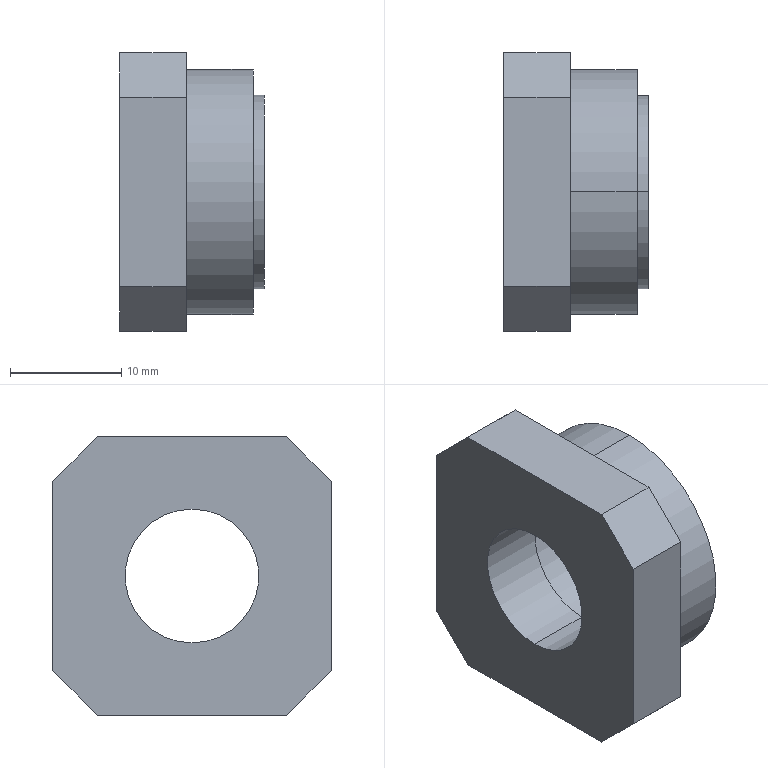Part | SolidWorks | features ICE 2, Chamfer 1, Extrusion 1, HoleWzd 1 | 1 solid | 21 faces | box 13 x 25 x 25 mm | volume 4305 mm3 | plane 13 | cylinder 8 | commonest cylinder face diameters 12 x2 14.1 x2 17.4 x2 22 x2
STEP:
#1=CARTESIAN_POINT('',(9.,0.,-8.7));
#2=VERTEX_POINT('',#1);
#3=CARTESIAN_POINT('',(9.,0.,8.7));
#4=VERTEX_POINT('',#3);
#5=CARTESIAN_POINT('',(9.,0.,0.));
#6=DIRECTION('',(1.,0.,0.));
#7=DIRECTION('',(0.,0.,-1.));
#8=AXIS2_PLACEMENT_3D('',#5,#6,#7);
#9=CIRCLE('',#8,8.7);
#10=EDGE_CURVE('',#2,#4,#9,.T.);
#11=ORIENTED_EDGE('',*,*,#10,.T.);
#12=CARTESIAN_POINT('',(10.,0.,8.7));
#13=VERTEX_POINT('',#12);
#14=CARTESIAN_POINT('',(9.,0.,8.7));
#15=DIRECTION('',(1.,0.,0.));
#16=VECTOR('',#15,1000.);
#17=LINE('',#14,#16);
#18=EDGE_CURVE('',#4,#13,#17,.T.);
#19=ORIENTED_EDGE('',*,*,#18,.T.);
#20=CARTESIAN_POINT('',(10.,0.,-8.7));
#21=VERTEX_POINT('',#20);
#22=CARTESIAN_POINT('',(10.,0.,0.));
#23=DIRECTION('',(1.,0.,0.));
#24=DIRECTION('',(0.,0.,-1.));
#25=AXIS2_PLACEMENT_3D('',#22,#23,#24);
#26=CIRCLE('',#25,8.7);
#27=EDGE_CURVE('',#21,#13,#26,.T.);
#28=ORIENTED_EDGE('',*,*,#27,.F.);
#29=CARTESIAN_POINT('',(9.,0.,-8.7));
#30=DIRECTION('',(1.,0.,0.));
#31=VECTOR('',#30,1000.);
#32=LINE('',#29,#31);
#33=EDGE_CURVE('',#2,#21,#32,.T.);
#34=ORIENTED_EDGE('',*,*,#33,.F.);
#35=EDGE_LOOP('',(#11,#19,#28,#34));
#36=FACE_OUTER_BOUND('',#35,.T.);
#37=CARTESIAN_POINT('',(9.,0.,0.));
#38=DIRECTION('',(1.,0.,0.));
#39=DIRECTION('',(0.,0.,-1.));
#40=AXIS2_PLACEMENT_3D('',#37,#38,#39);
#41=CYLINDRICAL_SURFACE('',#40,8.7);
#42=ADVANCED_FACE('',(#36),#41,.T.);
#43=CARTESIAN_POINT('',(10.,0.,7.05));
#44=VERTEX_POINT('',#43);
#45=CARTESIAN_POINT('',(10.,0.,-7.05));
#46=VERTEX_POINT('',#45);
#47=CARTESIAN_POINT('',(10.,0.,0.));
#48=DIRECTION('',(1.,0.,0.));
#49=DIRECTION('',(0.,0.,-1.));
#50=AXIS2_PLACEMENT_3D('',#47,#48,#49);
#51=CIRCLE('',#50,7.05);
#52=EDGE_CURVE('',#44,#46,#51,.T.);
#53=ORIENTED_EDGE('',*,*,#52,.T.);
#54=CARTESIAN_POINT('',(3.,0.,-7.05));
#55=VERTEX_POINT('',#54);
#56=CARTESIAN_POINT('',(10.,0.,-7.05));
#57=DIRECTION('',(-1.,0.,0.));
#58=VECTOR('',#57,1000.);
#59=LINE('',#56,#58);
#60=EDGE_CURVE('',#46,#55,#59,.T.);
#61=ORIENTED_EDGE('',*,*,#60,.T.);
#62=CARTESIAN_POINT('',(3.,0.,7.05));
#63=VERTEX_POINT('',#62);
#64=CARTESIAN_POINT('',(3.,0.,0.));
#65=DIRECTION('',(1.,0.,0.));
#66=DIRECTION('',(0.,0.,-1.));
#67=AXIS2_PLACEMENT_3D('',#64,#65,#66);
#68=CIRCLE('',#67,7.05);
#69=EDGE_CURVE('',#63,#55,#68,.T.);
#70=ORIENTED_EDGE('',*,*,#69,.F.);
#71=CARTESIAN_POINT('',(10.,0.,7.05));
#72=DIRECTION('',(-1.,0.,0.));
#73=VECTOR('',#72,1000.);
#74=LINE('',#71,#73);
#75=EDGE_CURVE('',#44,#63,#74,.T.);
#76=ORIENTED_EDGE('',*,*,#75,.F.);
#77=EDGE_LOOP('',(#53,#61,#70,#76));
#78=FACE_OUTER_BOUND('',#77,.T.);
#79=CARTESIAN_POINT('',(10.,0.,0.));
#80=DIRECTION('',(-1.,0.,0.));
#81=DIRECTION('',(0.,0.,1.));
#82=AXIS2_PLACEMENT_3D('',#79,#80,#81);
#83=CYLINDRICAL_SURFACE('',#82,7.05);
#84=ADVANCED_FACE('',(#78),#83,.F.);
#85=CARTESIAN_POINT('',(3.,0.,-6.));
#86=VERTEX_POINT('',#85);
#87=CARTESIAN_POINT('',(3.,0.,6.));
#88=VERTEX_POINT('',#87);
#89=CARTESIAN_POINT('',(3.,0.,0.));
#90=DIRECTION('',(-1.,0.,0.));
#91=DIRECTION('',(0.,0.,1.));
#92=AXIS2_PLACEMENT_3D('',#89,#90,#91);
#93=CIRCLE('',#92,6.);
#94=EDGE_CURVE('',#86,#88,#93,.T.);
#95=ORIENTED_EDGE('',*,*,#94,.F.);
#96=CARTESIAN_POINT('',(-3.,0.,-6.));
#97=VERTEX_POINT('',#96);
#98=CARTESIAN_POINT('',(-3.,0.,-6.));
#99=DIRECTION('',(-1.,0.,0.));
#100=VECTOR('',#99,1000.);
#101=LINE('',#98,#100);
#102=EDGE_CURVE('',#86,#97,#101,.T.);
#103=ORIENTED_EDGE('',*,*,#102,.T.);
#104=CARTESIAN_POINT('',(-3.,0.,6.));
#105=VERTEX_POINT('',#104);
#106=CARTESIAN_POINT('',(-3.,0.,0.));
#107=DIRECTION('',(-1.,0.,0.));
#108=DIRECTION('',(0.,0.,1.));
#109=AXIS2_PLACEMENT_3D('',#106,#107,#108);
#110=CIRCLE('',#109,6.);
#111=EDGE_CURVE('',#97,#105,#110,.T.);
#112=ORIENTED_EDGE('',*,*,#111,.T.);
#113=CARTESIAN_POINT('',(-3.,0.,6.));
#114=DIRECTION('',(-1.,0.,0.));
#115=VECTOR('',#114,1000.);
#116=LINE('',#113,#115);
#117=EDGE_CURVE('',#88,#105,#116,.T.);
#118=ORIENTED_EDGE('',*,*,#117,.F.);
#119=EDGE_LOOP('',(#95,#103,#112,#118));
#120=FACE_OUTER_BOUND('',#119,.T.);
#121=CARTESIAN_POINT('',(-3.,0.,0.));
#122=DIRECTION('',(-1.,0.,0.));
#123=DIRECTION('',(0.,0.,1.));
#124=AXIS2_PLACEMENT_3D('',#121,#122,#123);
#125=CYLINDRICAL_SURFACE('',#124,6.);
#126=ADVANCED_FACE('',(#120),#125,.F.);
#127=CARTESIAN_POINT('',(9.,0.,-11.));
#128=VERTEX_POINT('',#127);
#129=CARTESIAN_POINT('',(9.,0.,11.));
#130=VERTEX_POINT('',#129);
#131=CARTESIAN_POINT('',(9.,0.,0.));
#132=DIRECTION('',(1.,0.,0.));
#133=DIRECTION('',(0.,0.,-1.));
#134=AXIS2_PLACEMENT_3D('',#131,#132,#133);
#135=CIRCLE('',#134,11.);
#136=EDGE_CURVE('',#128,#130,#135,.T.);
#137=ORIENTED_EDGE('',*,*,#136,.F.);
#138=CARTESIAN_POINT('',(3.,0.,-11.));
#139=VERTEX_POINT('',#138);
#140=CARTESIAN_POINT('',(10.,0.,-11.));
#141=DIRECTION('',(-1.,0.,0.));
#142=VECTOR('',#141,1000.);
#143=LINE('',#140,#142);
#144=EDGE_CURVE('',#128,#139,#143,.T.);
#145=ORIENTED_EDGE('',*,*,#144,.T.);
#146=CARTESIAN_POINT('',(3.,0.,11.));
#147=VERTEX_POINT('',#146);
#148=CARTESIAN_POINT('',(3.,0.,0.));
#149=DIRECTION('',(1.,0.,0.));
#150=DIRECTION('',(0.,0.,-1.));
#151=AXIS2_PLACEMENT_3D('',#148,#149,#150);
#152=CIRCLE('',#151,11.);
#153=EDGE_CURVE('',#139,#147,#152,.T.);
#154=ORIENTED_EDGE('',*,*,#153,.T.);
#155=CARTESIAN_POINT('',(10.,0.,11.));
#156=DIRECTION('',(-1.,0.,0.));
#157=VECTOR('',#156,1000.);
#158=LINE('',#155,#157);
#159=EDGE_CURVE('',#130,#147,#158,.T.);
#160=ORIENTED_EDGE('',*,*,#159,.F.);
#161=EDGE_LOOP('',(#137,#145,#154,#160));
#162=FACE_OUTER_BOUND('',#161,.T.);
#163=CARTESIAN_POINT('',(10.,0.,0.));
#164=DIRECTION('',(-1.,0.,0.));
#165=DIRECTION('',(0.,0.,1.));
#166=AXIS2_PLACEMENT_3D('',#163,#164,#165);
#167=CYLINDRICAL_SURFACE('',#166,11.);
#168=ADVANCED_FACE('',(#162),#167,.T.);
#169=ORIENTED_EDGE('',*,*,#52,.F.);
#170=CARTESIAN_POINT('',(10.,0.,0.));
#171=DIRECTION('',(1.,0.,0.));
#172=DIRECTION('',(0.,0.,-1.));
#173=AXIS2_PLACEMENT_3D('',#170,#171,#172);
#174=CIRCLE('',#173,7.05);
#175=EDGE_CURVE('',#46,#44,#174,.T.);
#176=ORIENTED_EDGE('',*,*,#175,.F.);
#177=EDGE_LOOP('',(#169,#176));
#178=FACE_BOUND('',#177,.T.);
#179=ORIENTED_EDGE('',*,*,#27,.T.);
#180=CARTESIAN_POINT('',(10.,0.,0.));
#181=DIRECTION('',(1.,0.,0.));
#182=DIRECTION('',(0.,0.,-1.));
#183=AXIS2_PLACEMENT_3D('',#180,#181,#182);
#184=CIRCLE('',#183,8.7);
#185=EDGE_CURVE('',#13,#21,#184,.T.);
#186=ORIENTED_EDGE('',*,*,#185,.T.);
#187=EDGE_LOOP('',(#179,#186));
#188=FACE_OUTER_BOUND('',#187,.T.);
#189=CARTESIAN_POINT('',(10.,0.,0.));
#190=DIRECTION('',(1.,0.,0.));
#191=DIRECTION('',(0.,0.,-1.));
#192=AXIS2_PLACEMENT_3D('',#189,#190,#191);
#193=PLANE('',#192);
#194=ADVANCED_FACE('',(#178,#188),#193,.T.);
#195=ORIENTED_EDGE('',*,*,#144,.F.);
#196=CARTESIAN_POINT('',(9.,0.,0.));
#197=DIRECTION('',(1.,0.,0.));
#198=DIRECTION('',(0.,0.,-1.));
#199=AXIS2_PLACEMENT_3D('',#196,#197,#198);
#200=CIRCLE('',#199,11.);
#201=EDGE_CURVE('',#130,#128,#200,.T.);
#202=ORIENTED_EDGE('',*,*,#201,.F.);
#203=ORIENTED_EDGE('',*,*,#159,.T.);
#204=CARTESIAN_POINT('',(3.,0.,0.));
#205=DIRECTION('',(1.,0.,0.));
#206=DIRECTION('',(0.,0.,-1.));
#207=AXIS2_PLACEMENT_3D('',#204,#205,#206);
#208=CIRCLE('',#207,11.);
#209=EDGE_CURVE('',#147,#139,#208,.T.);
#210=ORIENTED_EDGE('',*,*,#209,.T.);
#211=EDGE_LOOP('',(#195,#202,#203,#210));
#212=FACE_OUTER_BOUND('',#211,.T.);
#213=CARTESIAN_POINT('',(10.,0.,0.));
#214=DIRECTION('',(-1.,0.,0.));
#215=DIRECTION('',(0.,0.,1.));
#216=AXIS2_PLACEMENT_3D('',#213,#214,#215);
#217=CYLINDRICAL_SURFACE('',#216,11.);
#218=ADVANCED_FACE('',(#212),#217,.T.);
#219=CARTESIAN_POINT('',(3.,0.,0.));
#220=DIRECTION('',(-1.,0.,0.));
#221=DIRECTION('',(0.,0.,1.));
#222=AXIS2_PLACEMENT_3D('',#219,#220,#221);
#223=CIRCLE('',#222,6.);
#224=EDGE_CURVE('',#88,#86,#223,.T.);
#225=ORIENTED_EDGE('',*,*,#224,.T.);
#226=ORIENTED_EDGE('',*,*,#94,.T.);
#227=EDGE_LOOP('',(#225,#226));
#228=FACE_BOUND('',#227,.T.);
#229=ORIENTED_EDGE('',*,*,#69,.T.);
#230=CARTESIAN_POINT('',(3.,0.,0.));
#231=DIRECTION('',(1.,0.,0.));
#232=DIRECTION('',(0.,0.,-1.));
#233=AXIS2_PLACEMENT_3D('',#230,#231,#232);
#234=CIRCLE('',#233,7.05);
#235=EDGE_CURVE('',#55,#63,#234,.T.);
#236=ORIENTED_EDGE('',*,*,#235,.T.);
#237=EDGE_LOOP('',(#229,#236));
#238=FACE_OUTER_BOUND('',#237,.T.);
#239=CARTESIAN_POINT('',(3.,0.,0.));
#240=DIRECTION('',(-1.,0.,0.));
#241=DIRECTION('',(0.,0.,1.));
#242=AXIS2_PLACEMENT_3D('',#239,#240,#241);
#243=PLANE('',#242);
#244=ADVANCED_FACE('',(#228,#238),#243,.F.);
#245=CARTESIAN_POINT('',(3.,-8.5,-12.5));
#246=VERTEX_POINT('',#245);
#247=CARTESIAN_POINT('',(3.,8.5,-12.5));
#248=VERTEX_POINT('',#247);
#249=CARTESIAN_POINT('',(3.,-12.5,-12.5));
#250=DIRECTION('',(0.,1.,0.));
#251=VECTOR('',#250,1000.);
#252=LINE('',#249,#251);
#253=EDGE_CURVE('',#246,#248,#252,.T.);
#254=ORIENTED_EDGE('',*,*,#253,.F.);
#255=CARTESIAN_POINT('',(-3.,-8.5,-12.5));
#256=VERTEX_POINT('',#255);
#257=CARTESIAN_POINT('',(3.,-8.5,-12.5));
#258=DIRECTION('',(-1.,0.,0.));
#259=VECTOR('',#258,1000.);
#260=LINE('',#257,#259);
#261=EDGE_CURVE('',#246,#256,#260,.T.);
#262=ORIENTED_EDGE('',*,*,#261,.T.);
#263=CARTESIAN_POINT('',(-3.,8.5,-12.5));
#264=VERTEX_POINT('',#263);
#265=CARTESIAN_POINT('',(-3.,-12.5,-12.5));
#266=DIRECTION('',(0.,1.,0.));
#267=VECTOR('',#266,1000.);
#268=LINE('',#265,#267);
#269=EDGE_CURVE('',#256,#264,#268,.T.);
#270=ORIENTED_EDGE('',*,*,#269,.T.);
#271=CARTESIAN_POINT('',(3.,8.5,-12.5));
#272=DIRECTION('',(1.,0.,0.));
#273=VECTOR('',#272,1000.);
#274=LINE('',#271,#273);
#275=EDGE_CURVE('',#264,#248,#274,.T.);
#276=ORIENTED_EDGE('',*,*,#275,.T.);
#277=EDGE_LOOP('',(#254,#262,#270,#276));
#278=FACE_OUTER_BOUND('',#277,.T.);
#279=CARTESIAN_POINT('',(3.,-12.5,-12.5));
#280=DIRECTION('',(0.,0.,1.));
#281=DIRECTION('',(1.,0.,0.));
#282=AXIS2_PLACEMENT_3D('',#279,#280,#281);
#283=PLANE('',#282);
#284=ADVANCED_FACE('',(#278),#283,.F.);
#285=CARTESIAN_POINT('',(3.,12.5,-8.5));
#286=VERTEX_POINT('',#285);
#287=CARTESIAN_POINT('',(3.,12.5,8.5));
#288=VERTEX_POINT('',#287);
#289=CARTESIAN_POINT('',(3.,12.5,12.5));
#290=DIRECTION('',(0.,0.,1.));
#291=VECTOR('',#290,1000.);
#292=LINE('',#289,#291);
#293=EDGE_CURVE('',#286,#288,#292,.T.);
#294=ORIENTED_EDGE('',*,*,#293,.F.);
#295=CARTESIAN_POINT('',(-3.,12.5,-8.5));
#296=VERTEX_POINT('',#295);
#297=CARTESIAN_POINT('',(3.,12.5,-8.5));
#298=DIRECTION('',(-1.,0.,0.));
#299=VECTOR('',#298,1000.);
#300=LINE('',#297,#299);
#301=EDGE_CURVE('',#286,#296,#300,.T.);
#302=ORIENTED_EDGE('',*,*,#301,.T.);
#303=CARTESIAN_POINT('',(-3.,12.5,8.5));
#304=VERTEX_POINT('',#303);
#305=CARTESIAN_POINT('',(-3.,12.5,12.5));
#306=DIRECTION('',(0.,0.,1.));
#307=VECTOR('',#306,1000.);
#308=LINE('',#305,#307);
#309=EDGE_CURVE('',#296,#304,#308,.T.);
#310=ORIENTED_EDGE('',*,*,#309,.T.);
#311=CARTESIAN_POINT('',(3.,12.5,8.5));
#312=DIRECTION('',(1.,0.,0.));
#313=VECTOR('',#312,1000.);
#314=LINE('',#311,#313);
#315=EDGE_CURVE('',#304,#288,#314,.T.);
#316=ORIENTED_EDGE('',*,*,#315,.T.);
#317=EDGE_LOOP('',(#294,#302,#310,#316));
#318=FACE_OUTER_BOUND('',#317,.T.);
#319=CARTESIAN_POINT('',(3.,12.5,12.5));
#320=DIRECTION('',(0.,-1.,0.));
#321=DIRECTION('',(0.,0.,-1.));
#322=AXIS2_PLACEMENT_3D('',#319,#320,#321);
#323=PLANE('',#322);
#324=ADVANCED_FACE('',(#318),#323,.F.);
#325=CARTESIAN_POINT('',(-3.,8.5,12.5));
#326=VERTEX_POINT('',#325);
#327=CARTESIAN_POINT('',(-3.,-8.5,12.5));
#328=VERTEX_POINT('',#327);
#329=CARTESIAN_POINT('',(-3.,-12.5,12.5));
#330=DIRECTION('',(0.,-1.,0.));
#331=VECTOR('',#330,1000.);
#332=LINE('',#329,#331);
#333=EDGE_CURVE('',#326,#328,#332,.T.);
#334=ORIENTED_EDGE('',*,*,#333,.T.);
#335=CARTESIAN_POINT('',(3.,-8.5,12.5));
#336=VERTEX_POINT('',#335);
#337=CARTESIAN_POINT('',(3.,-8.5,12.5));
#338=DIRECTION('',(1.,0.,0.));
#339=VECTOR('',#338,1000.);
#340=LINE('',#337,#339);
#341=EDGE_CURVE('',#328,#336,#340,.T.);
#342=ORIENTED_EDGE('',*,*,#341,.T.);
#343=CARTESIAN_POINT('',(3.,8.5,12.5));
#344=VERTEX_POINT('',#343);
#345=CARTESIAN_POINT('',(3.,-12.5,12.5));
#346=DIRECTION('',(0.,-1.,0.));
#347=VECTOR('',#346,1000.);
#348=LINE('',#345,#347);
#349=EDGE_CURVE('',#344,#336,#348,.T.);
#350=ORIENTED_EDGE('',*,*,#349,.F.);
#351=CARTESIAN_POINT('',(3.,8.5,12.5));
#352=DIRECTION('',(-1.,0.,0.));
#353=VECTOR('',#352,1000.);
#354=LINE('',#351,#353);
#355=EDGE_CURVE('',#344,#326,#354,.T.);
#356=ORIENTED_EDGE('',*,*,#355,.T.);
#357=EDGE_LOOP('',(#334,#342,#350,#356));
#358=FACE_OUTER_BOUND('',#357,.T.);
#359=CARTESIAN_POINT('',(3.,-12.5,12.5));
#360=DIRECTION('',(0.,0.,-1.));
#361=DIRECTION('',(-1.,0.,0.));
#362=AXIS2_PLACEMENT_3D('',#359,#360,#361);
#363=PLANE('',#362);
#364=ADVANCED_FACE('',(#358),#363,.F.);
#365=CARTESIAN_POINT('',(3.,-12.5,8.5));
#366=VERTEX_POINT('',#365);
#367=CARTESIAN_POINT('',(3.,-12.5,-8.5));
#368=VERTEX_POINT('',#367);
#369=CARTESIAN_POINT('',(3.,-12.5,12.5));
#370=DIRECTION('',(0.,0.,-1.));
#371=VECTOR('',#370,1000.);
#372=LINE('',#369,#371);
#373=EDGE_CURVE('',#366,#368,#372,.T.);
#374=ORIENTED_EDGE('',*,*,#373,.F.);
#375=CARTESIAN_POINT('',(-3.,-12.5,8.5));
#376=VERTEX_POINT('',#375);
#377=CARTESIAN_POINT('',(3.,-12.5,8.5));
#378=DIRECTION('',(-1.,0.,0.));
#379=VECTOR('',#378,1000.);
#380=LINE('',#377,#379);
#381=EDGE_CURVE('',#366,#376,#380,.T.);
#382=ORIENTED_EDGE('',*,*,#381,.T.);
#383=CARTESIAN_POINT('',(-3.,-12.5,-8.5));
#384=VERTEX_POINT('',#383);
#385=CARTESIAN_POINT('',(-3.,-12.5,12.5));
#386=DIRECTION('',(0.,0.,-1.));
#387=VECTOR('',#386,1000.);
#388=LINE('',#385,#387);
#389=EDGE_CURVE('',#376,#384,#388,.T.);
#390=ORIENTED_EDGE('',*,*,#389,.T.);
#391=CARTESIAN_POINT('',(3.,-12.5,-8.5));
#392=DIRECTION('',(1.,0.,0.));
#393=VECTOR('',#392,1000.);
#394=LINE('',#391,#393);
#395=EDGE_CURVE('',#384,#368,#394,.T.);
#396=ORIENTED_EDGE('',*,*,#395,.T.);
#397=EDGE_LOOP('',(#374,#382,#390,#396));
#398=FACE_OUTER_BOUND('',#397,.T.);
#399=CARTESIAN_POINT('',(3.,-12.5,12.5));
#400=DIRECTION('',(0.,1.,0.));
#401=DIRECTION('',(0.,0.,1.));
#402=AXIS2_PLACEMENT_3D('',#399,#400,#401);
#403=PLANE('',#402);
#404=ADVANCED_FACE('',(#398),#403,.F.);
#405=ORIENTED_EDGE('',*,*,#209,.F.);
#406=ORIENTED_EDGE('',*,*,#153,.F.);
#407=EDGE_LOOP('',(#405,#406));
#408=FACE_BOUND('',#407,.T.);
#409=ORIENTED_EDGE('',*,*,#349,.T.);
#410=CARTESIAN_POINT('',(3.,-12.5,8.5));
#411=DIRECTION('',(0.,-0.7071,-0.7071));
#412=VECTOR('',#411,1000.);
#413=LINE('',#410,#412);
#414=EDGE_CURVE('',#336,#366,#413,.T.);
#415=ORIENTED_EDGE('',*,*,#414,.T.);
#416=ORIENTED_EDGE('',*,*,#373,.T.);
#417=CARTESIAN_POINT('',(3.,-8.5,-12.5));
#418=DIRECTION('',(0.,0.7071,-0.7071));
#419=VECTOR('',#418,1000.);
#420=LINE('',#417,#419);
#421=EDGE_CURVE('',#368,#246,#420,.T.);
#422=ORIENTED_EDGE('',*,*,#421,.T.);
#423=ORIENTED_EDGE('',*,*,#253,.T.);
#424=CARTESIAN_POINT('',(3.,12.5,-8.5));
#425=DIRECTION('',(0.,0.7071,0.7071));
#426=VECTOR('',#425,1000.);
#427=LINE('',#424,#426);
#428=EDGE_CURVE('',#248,#286,#427,.T.);
#429=ORIENTED_EDGE('',*,*,#428,.T.);
#430=ORIENTED_EDGE('',*,*,#293,.T.);
#431=CARTESIAN_POINT('',(3.,8.5,12.5));
#432=DIRECTION('',(0.,-0.7071,0.7071));
#433=VECTOR('',#432,1000.);
#434=LINE('',#431,#433);
#435=EDGE_CURVE('',#288,#344,#434,.T.);
#436=ORIENTED_EDGE('',*,*,#435,.T.);
#437=EDGE_LOOP('',(#409,#415,#416,#422,#423,#429,#430,#436));
#438=FACE_OUTER_BOUND('',#437,.T.);
#439=CARTESIAN_POINT('',(3.,0.,0.));
#440=DIRECTION('',(-1.,0.,0.));
#441=DIRECTION('',(0.,0.,1.));
#442=AXIS2_PLACEMENT_3D('',#439,#440,#441);
#443=PLANE('',#442);
#444=ADVANCED_FACE('',(#408,#438),#443,.F.);
#445=CARTESIAN_POINT('',(-3.,0.,0.));
#446=DIRECTION('',(-1.,0.,0.));
#447=DIRECTION('',(0.,0.,1.));
#448=AXIS2_PLACEMENT_3D('',#445,#446,#447);
#449=CIRCLE('',#448,6.);
#450=EDGE_CURVE('',#105,#97,#449,.T.);
#451=ORIENTED_EDGE('',*,*,#450,.F.);
#452=ORIENTED_EDGE('',*,*,#111,.F.);
#453=EDGE_LOOP('',(#451,#452));
#454=FACE_BOUND('',#453,.T.);
#455=ORIENTED_EDGE('',*,*,#389,.F.);
#456=CARTESIAN_POINT('',(-3.,-10.5,10.5));
#457=DIRECTION('',(0.,0.7071,0.7071));
#458=VECTOR('',#457,1000.);
#459=LINE('',#456,#458);
#460=EDGE_CURVE('',#376,#328,#459,.T.);
#461=ORIENTED_EDGE('',*,*,#460,.T.);
#462=ORIENTED_EDGE('',*,*,#333,.F.);
#463=CARTESIAN_POINT('',(-3.,10.5,10.5));
#464=DIRECTION('',(0.,0.7071,-0.7071));
#465=VECTOR('',#464,1000.);
#466=LINE('',#463,#465);
#467=EDGE_CURVE('',#326,#304,#466,.T.);
#468=ORIENTED_EDGE('',*,*,#467,.T.);
#469=ORIENTED_EDGE('',*,*,#309,.F.);
#470=CARTESIAN_POINT('',(-3.,10.5,-10.5));
#471=DIRECTION('',(0.,-0.7071,-0.7071));
#472=VECTOR('',#471,1000.);
#473=LINE('',#470,#472);
#474=EDGE_CURVE('',#296,#264,#473,.T.);
#475=ORIENTED_EDGE('',*,*,#474,.T.);
#476=ORIENTED_EDGE('',*,*,#269,.F.);
#477=CARTESIAN_POINT('',(-3.,-10.5,-10.5));
#478=DIRECTION('',(0.,-0.7071,0.7071));
#479=VECTOR('',#478,1000.);
#480=LINE('',#477,#479);
#481=EDGE_CURVE('',#256,#384,#480,.T.);
#482=ORIENTED_EDGE('',*,*,#481,.T.);
#483=EDGE_LOOP('',(#455,#461,#462,#468,#469,#475,#476,#482));
#484=FACE_OUTER_BOUND('',#483,.T.);
#485=CARTESIAN_POINT('',(-3.,0.,0.));
#486=DIRECTION('',(-1.,0.,0.));
#487=DIRECTION('',(0.,0.,1.));
#488=AXIS2_PLACEMENT_3D('',#485,#486,#487);
#489=PLANE('',#488);
#490=ADVANCED_FACE('',(#454,#484),#489,.T.);
#491=ORIENTED_EDGE('',*,*,#102,.F.);
#492=ORIENTED_EDGE('',*,*,#224,.F.);
#493=ORIENTED_EDGE('',*,*,#117,.T.);
#494=ORIENTED_EDGE('',*,*,#450,.T.);
#495=EDGE_LOOP('',(#491,#492,#493,#494));
#496=FACE_OUTER_BOUND('',#495,.T.);
#497=CARTESIAN_POINT('',(-3.,0.,0.));
#498=DIRECTION('',(-1.,0.,0.));
#499=DIRECTION('',(0.,0.,1.));
#500=AXIS2_PLACEMENT_3D('',#497,#498,#499);
#501=CYLINDRICAL_SURFACE('',#500,6.);
#502=ADVANCED_FACE('',(#496),#501,.F.);
#503=ORIENTED_EDGE('',*,*,#60,.F.);
#504=ORIENTED_EDGE('',*,*,#175,.T.);
#505=ORIENTED_EDGE('',*,*,#75,.T.);
#506=ORIENTED_EDGE('',*,*,#235,.F.);
#507=EDGE_LOOP('',(#503,#504,#505,#506));
#508=FACE_OUTER_BOUND('',#507,.T.);
#509=CARTESIAN_POINT('',(10.,0.,0.));
#510=DIRECTION('',(-1.,0.,0.));
#511=DIRECTION('',(0.,0.,1.));
#512=AXIS2_PLACEMENT_3D('',#509,#510,#511);
#513=CYLINDRICAL_SURFACE('',#512,7.05);
#514=ADVANCED_FACE('',(#508),#513,.F.);
#515=ORIENTED_EDGE('',*,*,#10,.F.);
#516=CARTESIAN_POINT('',(9.,0.,0.));
#517=DIRECTION('',(1.,0.,0.));
#518=DIRECTION('',(0.,0.,-1.));
#519=AXIS2_PLACEMENT_3D('',#516,#517,#518);
#520=CIRCLE('',#519,8.7);
#521=EDGE_CURVE('',#4,#2,#520,.T.);
#522=ORIENTED_EDGE('',*,*,#521,.F.);
#523=EDGE_LOOP('',(#515,#522));
#524=FACE_BOUND('',#523,.T.);
#525=ORIENTED_EDGE('',*,*,#201,.T.);
#526=ORIENTED_EDGE('',*,*,#136,.T.);
#527=EDGE_LOOP('',(#525,#526));
#528=FACE_OUTER_BOUND('',#527,.T.);
#529=CARTESIAN_POINT('',(9.,0.,0.));
#530=DIRECTION('',(1.,0.,0.));
#531=DIRECTION('',(0.,0.,-1.));
#532=AXIS2_PLACEMENT_3D('',#529,#530,#531);
#533=PLANE('',#532);
#534=ADVANCED_FACE('',(#524,#528),#533,.T.);
#535=ORIENTED_EDGE('',*,*,#18,.F.);
#536=ORIENTED_EDGE('',*,*,#521,.T.);
#537=ORIENTED_EDGE('',*,*,#33,.T.);
#538=ORIENTED_EDGE('',*,*,#185,.F.);
#539=EDGE_LOOP('',(#535,#536,#537,#538));
#540=FACE_OUTER_BOUND('',#539,.T.);
#541=CARTESIAN_POINT('',(9.,0.,0.));
#542=DIRECTION('',(1.,0.,0.));
#543=DIRECTION('',(0.,0.,-1.));
#544=AXIS2_PLACEMENT_3D('',#541,#542,#543);
#545=CYLINDRICAL_SURFACE('',#544,8.7);
#546=ADVANCED_FACE('',(#540),#545,.T.);
#547=ORIENTED_EDGE('',*,*,#414,.F.);
#548=ORIENTED_EDGE('',*,*,#341,.F.);
#549=ORIENTED_EDGE('',*,*,#460,.F.);
#550=ORIENTED_EDGE('',*,*,#381,.F.);
#551=EDGE_LOOP('',(#547,#548,#549,#550));
#552=FACE_OUTER_BOUND('',#551,.T.);
#553=CARTESIAN_POINT('',(3.,-12.5,8.5));
#554=DIRECTION('',(0.,0.7071,-0.7071));
#555=DIRECTION('',(-1.,0.,0.));
#556=AXIS2_PLACEMENT_3D('',#553,#554,#555);
#557=PLANE('',#556);
#558=ADVANCED_FACE('',(#552),#557,.F.);
#559=ORIENTED_EDGE('',*,*,#421,.F.);
#560=ORIENTED_EDGE('',*,*,#395,.F.);
#561=ORIENTED_EDGE('',*,*,#481,.F.);
#562=ORIENTED_EDGE('',*,*,#261,.F.);
#563=EDGE_LOOP('',(#559,#560,#561,#562));
#564=FACE_OUTER_BOUND('',#563,.T.);
#565=CARTESIAN_POINT('',(3.,-8.5,-12.5));
#566=DIRECTION('',(0.,0.7071,0.7071));
#567=DIRECTION('',(-1.,0.,0.));
#568=AXIS2_PLACEMENT_3D('',#565,#566,#567);
#569=PLANE('',#568);
#570=ADVANCED_FACE('',(#564),#569,.F.);
#571=ORIENTED_EDGE('',*,*,#428,.F.);
#572=ORIENTED_EDGE('',*,*,#275,.F.);
#573=ORIENTED_EDGE('',*,*,#474,.F.);
#574=ORIENTED_EDGE('',*,*,#301,.F.);
#575=EDGE_LOOP('',(#571,#572,#573,#574));
#576=FACE_OUTER_BOUND('',#575,.T.);
#577=CARTESIAN_POINT('',(3.,12.5,-8.5));
#578=DIRECTION('',(0.,-0.7071,0.7071));
#579=DIRECTION('',(-1.,0.,0.));
#580=AXIS2_PLACEMENT_3D('',#577,#578,#579);
#581=PLANE('',#580);
#582=ADVANCED_FACE('',(#576),#581,.F.);
#583=ORIENTED_EDGE('',*,*,#435,.F.);
#584=ORIENTED_EDGE('',*,*,#315,.F.);
#585=ORIENTED_EDGE('',*,*,#467,.F.);
#586=ORIENTED_EDGE('',*,*,#355,.F.);
#587=EDGE_LOOP('',(#583,#584,#585,#586));
#588=FACE_OUTER_BOUND('',#587,.T.);
#589=CARTESIAN_POINT('',(3.,8.5,12.5));
#590=DIRECTION('',(0.,-0.7071,-0.7071));
#591=DIRECTION('',(-1.,0.,0.));
#592=AXIS2_PLACEMENT_3D('',#589,#590,#591);
#593=PLANE('',#592);
#594=ADVANCED_FACE('',(#588),#593,.F.);
#595=CLOSED_SHELL('',(#42,#84,#126,#168,#194,#218,#244,#284,#324,#364,#404,#444,#490,#502,#514,#534,#546,#558,#570,#582,#594));
#596=MANIFOLD_SOLID_BREP('',#595);
#597=CARTESIAN_POINT('',(0.,0.,0.));
#598=DIRECTION('',(0.,0.,1.));
#599=DIRECTION('',(1.,0.,0.));
#600=AXIS2_PLACEMENT_3D('',#597,#598,#599);
#601=(LENGTH_UNIT()NAMED_UNIT(*)SI_UNIT(.MILLI.,.METRE.));
#602=UNCERTAINTY_MEASURE_WITH_UNIT(LENGTH_MEASURE(0.00001),#601,'','');
#603=(NAMED_UNIT(*)PLANE_ANGLE_UNIT()SI_UNIT($,.RADIAN.));
#604=(NAMED_UNIT(*)SI_UNIT($,.STERADIAN.)SOLID_ANGLE_UNIT());
#605=(GEOMETRIC_REPRESENTATION_CONTEXT(3)GLOBAL_UNCERTAINTY_ASSIGNED_CONTEXT((#602))GLOBAL_UNIT_ASSIGNED_CONTEXT((#601,#603,#604))REPRESENTATION_CONTEXT('',''));
#606=ADVANCED_BREP_SHAPE_REPRESENTATION('',(#596,#600),#605);